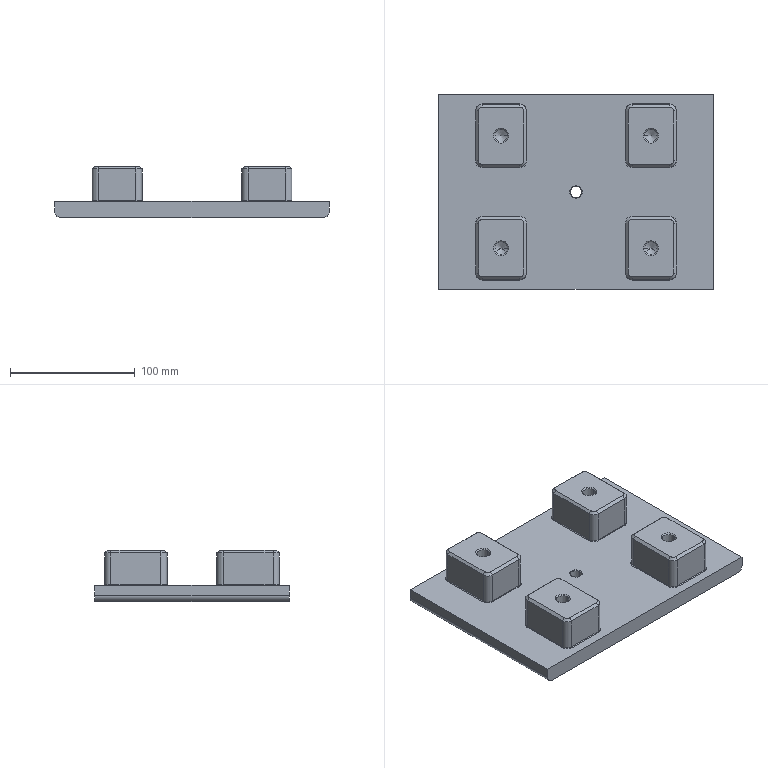Part | SolidWorks | features Fillet 4, ICE 3, 3DProfileFeature 2, HoleWzd 2, Chamfer 1, Extrusion 1 | 1 solid | 155 faces | box 220 x 156 x 41 mm | volume 648934 mm3 | cylinder 54 | plane 51 | cone 34 | torus 16 | commonest cylinder face diameters 10 x18 1 x16 10.2 x8 12 x6 2 x4 9 x2